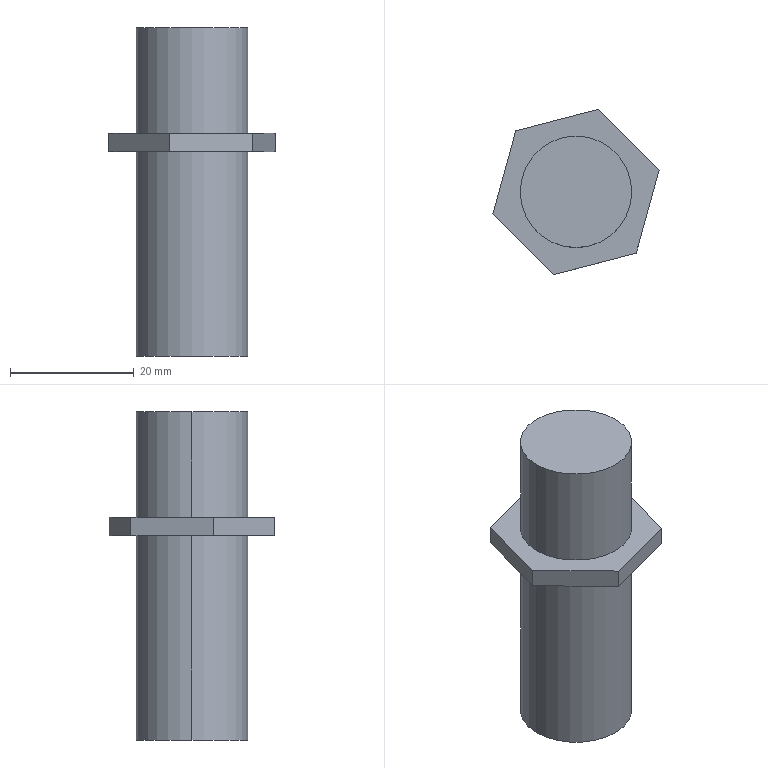Part | SolidWorks | features Extrusion 1, ICE 1 | 1 solid | 14 faces | box 26.811 x 26.725 x 53 mm | volume 14220 mm3 | plane 10 | cylinder 4 | commonest cylinder face diameters 18 x4
STEP:
#1=CARTESIAN_POINT('',(9.,0.,-33.));
#2=VERTEX_POINT('',#1);
#3=CARTESIAN_POINT('',(-9.,0.,-33.));
#4=VERTEX_POINT('',#3);
#5=CARTESIAN_POINT('',(0.,0.,-33.));
#6=DIRECTION('',(0.,0.,1.));
#7=DIRECTION('',(1.,0.,0.));
#8=AXIS2_PLACEMENT_3D('',#5,#6,#7);
#9=CIRCLE('',#8,9.);
#10=EDGE_CURVE('',#2,#4,#9,.T.);
#11=ORIENTED_EDGE('',*,*,#10,.T.);
#12=CARTESIAN_POINT('',(-9.,0.,0.));
#13=VERTEX_POINT('',#12);
#14=CARTESIAN_POINT('',(-9.,0.,-33.));
#15=DIRECTION('',(0.,0.,1.));
#16=VECTOR('',#15,1000.);
#17=LINE('',#14,#16);
#18=EDGE_CURVE('',#4,#13,#17,.T.);
#19=ORIENTED_EDGE('',*,*,#18,.T.);
#20=CARTESIAN_POINT('',(9.,0.,0.));
#21=VERTEX_POINT('',#20);
#22=CARTESIAN_POINT('',(0.,0.,0.));
#23=DIRECTION('',(0.,0.,-1.));
#24=DIRECTION('',(1.,0.,0.));
#25=AXIS2_PLACEMENT_3D('',#22,#23,#24);
#26=CIRCLE('',#25,9.);
#27=EDGE_CURVE('',#13,#21,#26,.T.);
#28=ORIENTED_EDGE('',*,*,#27,.T.);
#29=CARTESIAN_POINT('',(9.,0.,-33.));
#30=DIRECTION('',(0.,0.,1.));
#31=VECTOR('',#30,1000.);
#32=LINE('',#29,#31);
#33=EDGE_CURVE('',#2,#21,#32,.T.);
#34=ORIENTED_EDGE('',*,*,#33,.F.);
#35=EDGE_LOOP('',(#11,#19,#28,#34));
#36=FACE_OUTER_BOUND('',#35,.T.);
#37=CARTESIAN_POINT('',(0.,0.,-33.));
#38=DIRECTION('',(0.,0.,1.));
#39=DIRECTION('',(1.,0.,0.));
#40=AXIS2_PLACEMENT_3D('',#37,#38,#39);
#41=CYLINDRICAL_SURFACE('',#40,9.);
#42=ADVANCED_FACE('',(#36),#41,.T.);
#43=CARTESIAN_POINT('',(-9.,0.,3.));
#44=VERTEX_POINT('',#43);
#45=CARTESIAN_POINT('',(9.,0.,3.));
#46=VERTEX_POINT('',#45);
#47=CARTESIAN_POINT('',(0.,0.,3.));
#48=DIRECTION('',(0.,0.,-1.));
#49=DIRECTION('',(1.,0.,0.));
#50=AXIS2_PLACEMENT_3D('',#47,#48,#49);
#51=CIRCLE('',#50,9.);
#52=EDGE_CURVE('',#44,#46,#51,.T.);
#53=ORIENTED_EDGE('',*,*,#52,.F.);
#54=CARTESIAN_POINT('',(-9.,0.,20.));
#55=VERTEX_POINT('',#54);
#56=CARTESIAN_POINT('',(-9.,0.,-33.));
#57=DIRECTION('',(0.,0.,1.));
#58=VECTOR('',#57,1000.);
#59=LINE('',#56,#58);
#60=EDGE_CURVE('',#44,#55,#59,.T.);
#61=ORIENTED_EDGE('',*,*,#60,.T.);
#62=CARTESIAN_POINT('',(9.,0.,20.));
#63=VERTEX_POINT('',#62);
#64=CARTESIAN_POINT('',(0.,0.,20.));
#65=DIRECTION('',(0.,0.,1.));
#66=DIRECTION('',(1.,0.,0.));
#67=AXIS2_PLACEMENT_3D('',#64,#65,#66);
#68=CIRCLE('',#67,9.);
#69=EDGE_CURVE('',#63,#55,#68,.T.);
#70=ORIENTED_EDGE('',*,*,#69,.F.);
#71=CARTESIAN_POINT('',(9.,0.,-33.));
#72=DIRECTION('',(0.,0.,1.));
#73=VECTOR('',#72,1000.);
#74=LINE('',#71,#73);
#75=EDGE_CURVE('',#46,#63,#74,.T.);
#76=ORIENTED_EDGE('',*,*,#75,.F.);
#77=EDGE_LOOP('',(#53,#61,#70,#76));
#78=FACE_OUTER_BOUND('',#77,.T.);
#79=CARTESIAN_POINT('',(0.,0.,-33.));
#80=DIRECTION('',(0.,0.,1.));
#81=DIRECTION('',(1.,0.,0.));
#82=AXIS2_PLACEMENT_3D('',#79,#80,#81);
#83=CYLINDRICAL_SURFACE('',#82,9.);
#84=ADVANCED_FACE('',(#78),#83,.T.);
#85=ORIENTED_EDGE('',*,*,#60,.F.);
#86=CARTESIAN_POINT('',(0.,0.,3.));
#87=DIRECTION('',(0.,0.,-1.));
#88=DIRECTION('',(1.,0.,0.));
#89=AXIS2_PLACEMENT_3D('',#86,#87,#88);
#90=CIRCLE('',#89,9.);
#91=EDGE_CURVE('',#46,#44,#90,.T.);
#92=ORIENTED_EDGE('',*,*,#91,.F.);
#93=ORIENTED_EDGE('',*,*,#75,.T.);
#94=CARTESIAN_POINT('',(0.,0.,20.));
#95=DIRECTION('',(0.,0.,1.));
#96=DIRECTION('',(1.,0.,0.));
#97=AXIS2_PLACEMENT_3D('',#94,#95,#96);
#98=CIRCLE('',#97,9.);
#99=EDGE_CURVE('',#55,#63,#98,.T.);
#100=ORIENTED_EDGE('',*,*,#99,.F.);
#101=EDGE_LOOP('',(#85,#92,#93,#100));
#102=FACE_OUTER_BOUND('',#101,.T.);
#103=CARTESIAN_POINT('',(0.,0.,-33.));
#104=DIRECTION('',(0.,0.,1.));
#105=DIRECTION('',(1.,0.,0.));
#106=AXIS2_PLACEMENT_3D('',#103,#104,#105);
#107=CYLINDRICAL_SURFACE('',#106,9.);
#108=ADVANCED_FACE('',(#102),#107,.T.);
#109=ORIENTED_EDGE('',*,*,#69,.T.);
#110=ORIENTED_EDGE('',*,*,#99,.T.);
#111=EDGE_LOOP('',(#109,#110));
#112=FACE_OUTER_BOUND('',#111,.T.);
#113=CARTESIAN_POINT('',(0.,0.,20.));
#114=DIRECTION('',(0.,0.,1.));
#115=DIRECTION('',(1.,0.,0.));
#116=AXIS2_PLACEMENT_3D('',#113,#114,#115);
#117=PLANE('',#116);
#118=ADVANCED_FACE('',(#112),#117,.T.);
#119=CARTESIAN_POINT('',(-3.667,-13.362,0.));
#120=VERTEX_POINT('',#119);
#121=CARTESIAN_POINT('',(9.738,-9.857,0.));
#122=VERTEX_POINT('',#121);
#123=CARTESIAN_POINT('',(-3.667,-13.362,0.));
#124=DIRECTION('',(0.9675,0.253,0.));
#125=VECTOR('',#124,1000.);
#126=LINE('',#123,#125);
#127=EDGE_CURVE('',#120,#122,#126,.T.);
#128=ORIENTED_EDGE('',*,*,#127,.T.);
#129=CARTESIAN_POINT('',(9.738,-9.857,3.));
#130=VERTEX_POINT('',#129);
#131=CARTESIAN_POINT('',(9.738,-9.857,3.));
#132=DIRECTION('',(0.,0.,-1.));
#133=VECTOR('',#132,1000.);
#134=LINE('',#131,#133);
#135=EDGE_CURVE('',#130,#122,#134,.T.);
#136=ORIENTED_EDGE('',*,*,#135,.F.);
#137=CARTESIAN_POINT('',(-3.667,-13.362,3.));
#138=VERTEX_POINT('',#137);
#139=CARTESIAN_POINT('',(-3.667,-13.362,3.));
#140=DIRECTION('',(0.9675,0.253,0.));
#141=VECTOR('',#140,1000.);
#142=LINE('',#139,#141);
#143=EDGE_CURVE('',#138,#130,#142,.T.);
#144=ORIENTED_EDGE('',*,*,#143,.F.);
#145=CARTESIAN_POINT('',(-3.667,-13.362,3.));
#146=DIRECTION('',(0.,0.,-1.));
#147=VECTOR('',#146,1000.);
#148=LINE('',#145,#147);
#149=EDGE_CURVE('',#138,#120,#148,.T.);
#150=ORIENTED_EDGE('',*,*,#149,.T.);
#151=EDGE_LOOP('',(#128,#136,#144,#150));
#152=FACE_OUTER_BOUND('',#151,.T.);
#153=CARTESIAN_POINT('',(-3.667,-13.362,3.));
#154=DIRECTION('',(-0.253,0.9675,0.));
#155=DIRECTION('',(-0.9675,-0.253,0.));
#156=AXIS2_PLACEMENT_3D('',#153,#154,#155);
#157=PLANE('',#156);
#158=ADVANCED_FACE('',(#152),#157,.F.);
#159=CARTESIAN_POINT('',(13.406,3.505,0.));
#160=VERTEX_POINT('',#159);
#161=CARTESIAN_POINT('',(9.738,-9.857,0.));
#162=DIRECTION('',(0.2647,0.9643,0.));
#163=VECTOR('',#162,1000.);
#164=LINE('',#161,#163);
#165=EDGE_CURVE('',#122,#160,#164,.T.);
#166=ORIENTED_EDGE('',*,*,#165,.T.);
#167=CARTESIAN_POINT('',(13.406,3.505,3.));
#168=VERTEX_POINT('',#167);
#169=CARTESIAN_POINT('',(13.406,3.505,3.));
#170=DIRECTION('',(0.,0.,-1.));
#171=VECTOR('',#170,1000.);
#172=LINE('',#169,#171);
#173=EDGE_CURVE('',#168,#160,#172,.T.);
#174=ORIENTED_EDGE('',*,*,#173,.F.);
#175=CARTESIAN_POINT('',(9.738,-9.857,3.));
#176=DIRECTION('',(0.2647,0.9643,0.));
#177=VECTOR('',#176,1000.);
#178=LINE('',#175,#177);
#179=EDGE_CURVE('',#130,#168,#178,.T.);
#180=ORIENTED_EDGE('',*,*,#179,.F.);
#181=ORIENTED_EDGE('',*,*,#135,.T.);
#182=EDGE_LOOP('',(#166,#174,#180,#181));
#183=FACE_OUTER_BOUND('',#182,.T.);
#184=CARTESIAN_POINT('',(9.738,-9.857,3.));
#185=DIRECTION('',(-0.9643,0.2647,0.));
#186=DIRECTION('',(-0.2647,-0.9643,0.));
#187=AXIS2_PLACEMENT_3D('',#184,#185,#186);
#188=PLANE('',#187);
#189=ADVANCED_FACE('',(#183),#188,.F.);
#190=CARTESIAN_POINT('',(3.667,13.362,0.));
#191=VERTEX_POINT('',#190);
#192=CARTESIAN_POINT('',(13.406,3.505,0.));
#193=DIRECTION('',(-0.7028,0.7114,0.));
#194=VECTOR('',#193,1000.);
#195=LINE('',#192,#194);
#196=EDGE_CURVE('',#160,#191,#195,.T.);
#197=ORIENTED_EDGE('',*,*,#196,.T.);
#198=CARTESIAN_POINT('',(3.667,13.362,3.));
#199=VERTEX_POINT('',#198);
#200=CARTESIAN_POINT('',(3.667,13.362,3.));
#201=DIRECTION('',(0.,0.,-1.));
#202=VECTOR('',#201,1000.);
#203=LINE('',#200,#202);
#204=EDGE_CURVE('',#199,#191,#203,.T.);
#205=ORIENTED_EDGE('',*,*,#204,.F.);
#206=CARTESIAN_POINT('',(13.406,3.505,3.));
#207=DIRECTION('',(-0.7028,0.7114,0.));
#208=VECTOR('',#207,1000.);
#209=LINE('',#206,#208);
#210=EDGE_CURVE('',#168,#199,#209,.T.);
#211=ORIENTED_EDGE('',*,*,#210,.F.);
#212=ORIENTED_EDGE('',*,*,#173,.T.);
#213=EDGE_LOOP('',(#197,#205,#211,#212));
#214=FACE_OUTER_BOUND('',#213,.T.);
#215=CARTESIAN_POINT('',(13.406,3.505,3.));
#216=DIRECTION('',(-0.7114,-0.7028,0.));
#217=DIRECTION('',(0.7028,-0.7114,0.));
#218=AXIS2_PLACEMENT_3D('',#215,#216,#217);
#219=PLANE('',#218);
#220=ADVANCED_FACE('',(#214),#219,.F.);
#221=CARTESIAN_POINT('',(-9.738,9.857,0.));
#222=VERTEX_POINT('',#221);
#223=CARTESIAN_POINT('',(3.667,13.362,0.));
#224=DIRECTION('',(-0.9675,-0.253,0.));
#225=VECTOR('',#224,1000.);
#226=LINE('',#223,#225);
#227=EDGE_CURVE('',#191,#222,#226,.T.);
#228=ORIENTED_EDGE('',*,*,#227,.T.);
#229=CARTESIAN_POINT('',(-9.738,9.857,3.));
#230=VERTEX_POINT('',#229);
#231=CARTESIAN_POINT('',(-9.738,9.857,3.));
#232=DIRECTION('',(0.,0.,-1.));
#233=VECTOR('',#232,1000.);
#234=LINE('',#231,#233);
#235=EDGE_CURVE('',#230,#222,#234,.T.);
#236=ORIENTED_EDGE('',*,*,#235,.F.);
#237=CARTESIAN_POINT('',(3.667,13.362,3.));
#238=DIRECTION('',(-0.9675,-0.253,0.));
#239=VECTOR('',#238,1000.);
#240=LINE('',#237,#239);
#241=EDGE_CURVE('',#199,#230,#240,.T.);
#242=ORIENTED_EDGE('',*,*,#241,.F.);
#243=ORIENTED_EDGE('',*,*,#204,.T.);
#244=EDGE_LOOP('',(#228,#236,#242,#243));
#245=FACE_OUTER_BOUND('',#244,.T.);
#246=CARTESIAN_POINT('',(3.667,13.362,3.));
#247=DIRECTION('',(0.253,-0.9675,0.));
#248=DIRECTION('',(0.9675,0.253,0.));
#249=AXIS2_PLACEMENT_3D('',#246,#247,#248);
#250=PLANE('',#249);
#251=ADVANCED_FACE('',(#245),#250,.F.);
#252=CARTESIAN_POINT('',(-13.406,-3.505,0.));
#253=VERTEX_POINT('',#252);
#254=CARTESIAN_POINT('',(-9.738,9.857,0.));
#255=DIRECTION('',(-0.2647,-0.9643,0.));
#256=VECTOR('',#255,1000.);
#257=LINE('',#254,#256);
#258=EDGE_CURVE('',#222,#253,#257,.T.);
#259=ORIENTED_EDGE('',*,*,#258,.T.);
#260=CARTESIAN_POINT('',(-13.406,-3.505,3.));
#261=VERTEX_POINT('',#260);
#262=CARTESIAN_POINT('',(-13.406,-3.505,3.));
#263=DIRECTION('',(0.,0.,-1.));
#264=VECTOR('',#263,1000.);
#265=LINE('',#262,#264);
#266=EDGE_CURVE('',#261,#253,#265,.T.);
#267=ORIENTED_EDGE('',*,*,#266,.F.);
#268=CARTESIAN_POINT('',(-9.738,9.857,3.));
#269=DIRECTION('',(-0.2647,-0.9643,0.));
#270=VECTOR('',#269,1000.);
#271=LINE('',#268,#270);
#272=EDGE_CURVE('',#230,#261,#271,.T.);
#273=ORIENTED_EDGE('',*,*,#272,.F.);
#274=ORIENTED_EDGE('',*,*,#235,.T.);
#275=EDGE_LOOP('',(#259,#267,#273,#274));
#276=FACE_OUTER_BOUND('',#275,.T.);
#277=CARTESIAN_POINT('',(-9.738,9.857,3.));
#278=DIRECTION('',(0.9643,-0.2647,0.));
#279=DIRECTION('',(0.2647,0.9643,0.));
#280=AXIS2_PLACEMENT_3D('',#277,#278,#279);
#281=PLANE('',#280);
#282=ADVANCED_FACE('',(#276),#281,.F.);
#283=CARTESIAN_POINT('',(-13.406,-3.505,0.));
#284=DIRECTION('',(0.7028,-0.7114,0.));
#285=VECTOR('',#284,1000.);
#286=LINE('',#283,#285);
#287=EDGE_CURVE('',#253,#120,#286,.T.);
#288=ORIENTED_EDGE('',*,*,#287,.T.);
#289=ORIENTED_EDGE('',*,*,#149,.F.);
#290=CARTESIAN_POINT('',(-13.406,-3.505,3.));
#291=DIRECTION('',(0.7028,-0.7114,0.));
#292=VECTOR('',#291,1000.);
#293=LINE('',#290,#292);
#294=EDGE_CURVE('',#261,#138,#293,.T.);
#295=ORIENTED_EDGE('',*,*,#294,.F.);
#296=ORIENTED_EDGE('',*,*,#266,.T.);
#297=EDGE_LOOP('',(#288,#289,#295,#296));
#298=FACE_OUTER_BOUND('',#297,.T.);
#299=CARTESIAN_POINT('',(-13.406,-3.505,3.));
#300=DIRECTION('',(0.7114,0.7028,0.));
#301=DIRECTION('',(-0.7028,0.7114,0.));
#302=AXIS2_PLACEMENT_3D('',#299,#300,#301);
#303=PLANE('',#302);
#304=ADVANCED_FACE('',(#298),#303,.F.);
#305=ORIENTED_EDGE('',*,*,#91,.T.);
#306=ORIENTED_EDGE('',*,*,#52,.T.);
#307=EDGE_LOOP('',(#305,#306));
#308=FACE_BOUND('',#307,.T.);
#309=ORIENTED_EDGE('',*,*,#143,.T.);
#310=ORIENTED_EDGE('',*,*,#179,.T.);
#311=ORIENTED_EDGE('',*,*,#210,.T.);
#312=ORIENTED_EDGE('',*,*,#241,.T.);
#313=ORIENTED_EDGE('',*,*,#272,.T.);
#314=ORIENTED_EDGE('',*,*,#294,.T.);
#315=EDGE_LOOP('',(#309,#310,#311,#312,#313,#314));
#316=FACE_OUTER_BOUND('',#315,.T.);
#317=CARTESIAN_POINT('',(0.,0.,3.));
#318=DIRECTION('',(0.,0.,1.));
#319=DIRECTION('',(1.,0.,0.));
#320=AXIS2_PLACEMENT_3D('',#317,#318,#319);
#321=PLANE('',#320);
#322=ADVANCED_FACE('',(#308,#316),#321,.T.);
#323=CARTESIAN_POINT('',(0.,0.,0.));
#324=DIRECTION('',(0.,0.,-1.));
#325=DIRECTION('',(1.,0.,0.));
#326=AXIS2_PLACEMENT_3D('',#323,#324,#325);
#327=CIRCLE('',#326,9.);
#328=EDGE_CURVE('',#21,#13,#327,.T.);
#329=ORIENTED_EDGE('',*,*,#328,.F.);
#330=ORIENTED_EDGE('',*,*,#27,.F.);
#331=EDGE_LOOP('',(#329,#330));
#332=FACE_BOUND('',#331,.T.);
#333=ORIENTED_EDGE('',*,*,#127,.F.);
#334=ORIENTED_EDGE('',*,*,#287,.F.);
#335=ORIENTED_EDGE('',*,*,#258,.F.);
#336=ORIENTED_EDGE('',*,*,#227,.F.);
#337=ORIENTED_EDGE('',*,*,#196,.F.);
#338=ORIENTED_EDGE('',*,*,#165,.F.);
#339=EDGE_LOOP('',(#333,#334,#335,#336,#337,#338));
#340=FACE_OUTER_BOUND('',#339,.T.);
#341=CARTESIAN_POINT('',(0.,0.,0.));
#342=DIRECTION('',(0.,0.,1.));
#343=DIRECTION('',(1.,0.,0.));
#344=AXIS2_PLACEMENT_3D('',#341,#342,#343);
#345=PLANE('',#344);
#346=ADVANCED_FACE('',(#332,#340),#345,.F.);
#347=ORIENTED_EDGE('',*,*,#10,.F.);
#348=CARTESIAN_POINT('',(0.,0.,-33.));
#349=DIRECTION('',(0.,0.,1.));
#350=DIRECTION('',(1.,0.,0.));
#351=AXIS2_PLACEMENT_3D('',#348,#349,#350);
#352=CIRCLE('',#351,9.);
#353=EDGE_CURVE('',#4,#2,#352,.T.);
#354=ORIENTED_EDGE('',*,*,#353,.F.);
#355=EDGE_LOOP('',(#347,#354));
#356=FACE_OUTER_BOUND('',#355,.T.);
#357=CARTESIAN_POINT('',(0.,0.,-33.));
#358=DIRECTION('',(0.,0.,1.));
#359=DIRECTION('',(1.,0.,0.));
#360=AXIS2_PLACEMENT_3D('',#357,#358,#359);
#361=PLANE('',#360);
#362=ADVANCED_FACE('',(#356),#361,.F.);
#363=ORIENTED_EDGE('',*,*,#18,.F.);
#364=ORIENTED_EDGE('',*,*,#353,.T.);
#365=ORIENTED_EDGE('',*,*,#33,.T.);
#366=ORIENTED_EDGE('',*,*,#328,.T.);
#367=EDGE_LOOP('',(#363,#364,#365,#366));
#368=FACE_OUTER_BOUND('',#367,.T.);
#369=CARTESIAN_POINT('',(0.,0.,-33.));
#370=DIRECTION('',(0.,0.,1.));
#371=DIRECTION('',(1.,0.,0.));
#372=AXIS2_PLACEMENT_3D('',#369,#370,#371);
#373=CYLINDRICAL_SURFACE('',#372,9.);
#374=ADVANCED_FACE('',(#368),#373,.T.);
#375=CLOSED_SHELL('',(#42,#84,#108,#118,#158,#189,#220,#251,#282,#304,#322,#346,#362,#374));
#376=MANIFOLD_SOLID_BREP('',#375);
#377=CARTESIAN_POINT('',(0.,0.,0.));
#378=DIRECTION('',(0.,0.,1.));
#379=DIRECTION('',(1.,0.,0.));
#380=AXIS2_PLACEMENT_3D('',#377,#378,#379);
#381=(LENGTH_UNIT()NAMED_UNIT(*)SI_UNIT(.MILLI.,.METRE.));
#382=UNCERTAINTY_MEASURE_WITH_UNIT(LENGTH_MEASURE(0.00001),#381,'','');
#383=(NAMED_UNIT(*)PLANE_ANGLE_UNIT()SI_UNIT($,.RADIAN.));
#384=(NAMED_UNIT(*)SI_UNIT($,.STERADIAN.)SOLID_ANGLE_UNIT());
#385=(GEOMETRIC_REPRESENTATION_CONTEXT(3)GLOBAL_UNCERTAINTY_ASSIGNED_CONTEXT((#382))GLOBAL_UNIT_ASSIGNED_CONTEXT((#381,#383,#384))REPRESENTATION_CONTEXT('',''));
#386=ADVANCED_BREP_SHAPE_REPRESENTATION('',(#376,#380),#385);